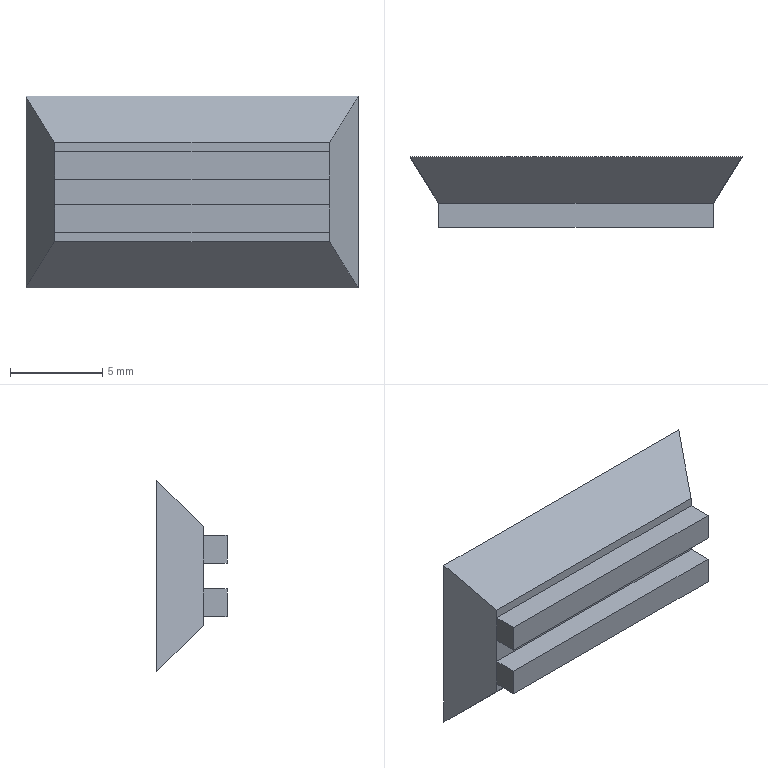Part | STEP file | D4NS_1CF_CAP^D4NS_1CF_Laser guard | 1 solid | 18 faces | box 18 x 3.8 x 10.4 mm | volume 386.227 mm3 | plane 18
STEP:
#1=CARTESIAN_POINT('',(0.,0.,0.));
#2=DIRECTION('',(0.,0.,1.));
#3=DIRECTION('',(1.,0.,0.));
#4=AXIS2_PLACEMENT_3D('',#1,#2,#3);
#5=CARTESIAN_POINT('',(-1.55,-3.8,7.4));
#6=VERTEX_POINT('',#5);
#7=CARTESIAN_POINT('',(-16.45,-3.8,7.4));
#8=VERTEX_POINT('',#7);
#9=CARTESIAN_POINT('',(-16.45,-3.8,7.4));
#10=DIRECTION('',(-1.,0.,0.));
#11=VECTOR('',#10,1.);
#12=LINE('',#9,#11);
#13=CARTESIAN_POINT('',(-1.55,-3.8,7.4));
#14=DIRECTION('',(0.,1.,0.));
#15=DIRECTION('',(1.,0.,0.));
#16=AXIS2_PLACEMENT_3D('',#13,#14,#15);
#17=PLANE('',#16);
#18=CARTESIAN_POINT('',(-14.9,0.));
#19=DIRECTION('',(-1.,0.));
#20=VECTOR('',#19,1.);
#21=LINE('',#18,#20);
#22=(GEOMETRIC_REPRESENTATION_CONTEXT(2)PARAMETRIC_REPRESENTATION_CONTEXT()REPRESENTATION_CONTEXT('',''));
#23=DEFINITIONAL_REPRESENTATION('',(#21),#22);
#24=PCURVE('',#17,#23);
#25=CARTESIAN_POINT('',(-16.45,-3.8,7.4));
#26=DIRECTION('',(0.,0.,-1.));
#27=DIRECTION('',(0.,-1.,0.));
#28=AXIS2_PLACEMENT_3D('',#25,#26,#27);
#29=PLANE('',#28);
#30=CARTESIAN_POINT('',(0.,0.));
#31=DIRECTION('',(0.,1.));
#32=VECTOR('',#31,1.);
#33=LINE('',#30,#32);
#34=(GEOMETRIC_REPRESENTATION_CONTEXT(2)PARAMETRIC_REPRESENTATION_CONTEXT()REPRESENTATION_CONTEXT('',''));
#35=DEFINITIONAL_REPRESENTATION('',(#33),#34);
#36=PCURVE('',#29,#35);
#37=SURFACE_CURVE('',#12,(#24,#36),.PCURVE_S1.);
#38=EDGE_CURVE('',#6,#8,#37,.T.);
#39=ORIENTED_EDGE('',*,*,#38,.T.);
#40=CARTESIAN_POINT('',(-16.45,-3.8,5.9));
#41=VERTEX_POINT('',#40);
#42=CARTESIAN_POINT('',(-16.45,-3.8,7.4));
#43=DIRECTION('',(0.,0.,-1.));
#44=VECTOR('',#43,1.);
#45=LINE('',#42,#44);
#46=CARTESIAN_POINT('',(-14.9,0.));
#47=DIRECTION('',(0.,1.));
#48=VECTOR('',#47,1.);
#49=LINE('',#46,#48);
#50=(GEOMETRIC_REPRESENTATION_CONTEXT(2)PARAMETRIC_REPRESENTATION_CONTEXT()REPRESENTATION_CONTEXT('',''));
#51=DEFINITIONAL_REPRESENTATION('',(#49),#50);
#52=PCURVE('',#17,#51);
#53=CARTESIAN_POINT('',(-16.45,-3.8,7.4));
#54=DIRECTION('',(1.,0.,0.));
#55=DIRECTION('',(0.,1.,0.));
#56=AXIS2_PLACEMENT_3D('',#53,#54,#55);
#57=PLANE('',#56);
#58=CARTESIAN_POINT('',(0.,0.));
#59=DIRECTION('',(0.,-1.));
#60=VECTOR('',#59,1.);
#61=LINE('',#58,#60);
#62=(GEOMETRIC_REPRESENTATION_CONTEXT(2)PARAMETRIC_REPRESENTATION_CONTEXT()REPRESENTATION_CONTEXT('',''));
#63=DEFINITIONAL_REPRESENTATION('',(#61),#62);
#64=PCURVE('',#57,#63);
#65=SURFACE_CURVE('',#45,(#52,#64),.PCURVE_S1.);
#66=EDGE_CURVE('',#8,#41,#65,.T.);
#67=ORIENTED_EDGE('',*,*,#66,.T.);
#68=CARTESIAN_POINT('',(-1.55,-3.8,5.9));
#69=VERTEX_POINT('',#68);
#70=CARTESIAN_POINT('',(-16.45,-3.8,5.9));
#71=DIRECTION('',(1.,0.,0.));
#72=VECTOR('',#71,1.);
#73=LINE('',#70,#72);
#74=CARTESIAN_POINT('',(-14.9,1.5));
#75=DIRECTION('',(1.,0.));
#76=VECTOR('',#75,1.);
#77=LINE('',#74,#76);
#78=(GEOMETRIC_REPRESENTATION_CONTEXT(2)PARAMETRIC_REPRESENTATION_CONTEXT()REPRESENTATION_CONTEXT('',''));
#79=DEFINITIONAL_REPRESENTATION('',(#77),#78);
#80=PCURVE('',#17,#79);
#81=CARTESIAN_POINT('',(-16.45,-3.8,5.9));
#82=DIRECTION('',(0.,0.,1.));
#83=DIRECTION('',(1.,0.,0.));
#84=AXIS2_PLACEMENT_3D('',#81,#82,#83);
#85=PLANE('',#84);
#86=CARTESIAN_POINT('',(0.,0.));
#87=DIRECTION('',(1.,0.));
#88=VECTOR('',#87,1.);
#89=LINE('',#86,#88);
#90=(GEOMETRIC_REPRESENTATION_CONTEXT(2)PARAMETRIC_REPRESENTATION_CONTEXT()REPRESENTATION_CONTEXT('',''));
#91=DEFINITIONAL_REPRESENTATION('',(#89),#90);
#92=PCURVE('',#85,#91);
#93=SURFACE_CURVE('',#73,(#80,#92),.PCURVE_S1.);
#94=EDGE_CURVE('',#41,#69,#93,.T.);
#95=ORIENTED_EDGE('',*,*,#94,.T.);
#96=CARTESIAN_POINT('',(-1.55,-3.8,7.4));
#97=DIRECTION('',(0.,0.,1.));
#98=VECTOR('',#97,1.);
#99=LINE('',#96,#98);
#100=CARTESIAN_POINT('',(0.,0.));
#101=DIRECTION('',(0.,-1.));
#102=VECTOR('',#101,1.);
#103=LINE('',#100,#102);
#104=(GEOMETRIC_REPRESENTATION_CONTEXT(2)PARAMETRIC_REPRESENTATION_CONTEXT()REPRESENTATION_CONTEXT('',''));
#105=DEFINITIONAL_REPRESENTATION('',(#103),#104);
#106=PCURVE('',#17,#105);
#107=CARTESIAN_POINT('',(-1.55,-3.8,7.4));
#108=DIRECTION('',(-1.,0.,0.));
#109=DIRECTION('',(0.,0.,1.));
#110=AXIS2_PLACEMENT_3D('',#107,#108,#109);
#111=PLANE('',#110);
#112=CARTESIAN_POINT('',(0.,0.));
#113=DIRECTION('',(1.,0.));
#114=VECTOR('',#113,1.);
#115=LINE('',#112,#114);
#116=(GEOMETRIC_REPRESENTATION_CONTEXT(2)PARAMETRIC_REPRESENTATION_CONTEXT()REPRESENTATION_CONTEXT('',''));
#117=DEFINITIONAL_REPRESENTATION('',(#115),#116);
#118=PCURVE('',#111,#117);
#119=SURFACE_CURVE('',#99,(#106,#118),.PCURVE_S1.);
#120=EDGE_CURVE('',#69,#6,#119,.T.);
#121=ORIENTED_EDGE('',*,*,#120,.T.);
#122=EDGE_LOOP('',(#39,#67,#95,#121));
#123=FACE_BOUND('',#122,.T.);
#124=ADVANCED_FACE('',(#123),#17,.F.);
#125=CARTESIAN_POINT('',(-1.55,-2.5,7.4));
#126=VERTEX_POINT('',#125);
#127=CARTESIAN_POINT('',(-16.45,-2.5,7.4));
#128=VERTEX_POINT('',#127);
#129=CARTESIAN_POINT('',(-16.45,-2.5,7.4));
#130=DIRECTION('',(-1.,0.,0.));
#131=VECTOR('',#130,1.);
#132=LINE('',#129,#131);
#133=CARTESIAN_POINT('',(-1.3,0.));
#134=DIRECTION('',(0.,1.));
#135=VECTOR('',#134,1.);
#136=LINE('',#133,#135);
#137=(GEOMETRIC_REPRESENTATION_CONTEXT(2)PARAMETRIC_REPRESENTATION_CONTEXT()REPRESENTATION_CONTEXT('',''));
#138=DEFINITIONAL_REPRESENTATION('',(#136),#137);
#139=PCURVE('',#29,#138);
#140=CARTESIAN_POINT('',(0.,-2.5,0.));
#141=DIRECTION('',(0.,-1.,0.));
#142=DIRECTION('',(0.,0.,-1.));
#143=AXIS2_PLACEMENT_3D('',#140,#141,#142);
#144=PLANE('',#143);
#145=CARTESIAN_POINT('',(-7.4,-16.45));
#146=DIRECTION('',(0.,-1.));
#147=VECTOR('',#146,1.);
#148=LINE('',#145,#147);
#149=(GEOMETRIC_REPRESENTATION_CONTEXT(2)PARAMETRIC_REPRESENTATION_CONTEXT()REPRESENTATION_CONTEXT('',''));
#150=DEFINITIONAL_REPRESENTATION('',(#148),#149);
#151=PCURVE('',#144,#150);
#152=SURFACE_CURVE('',#132,(#139,#151),.PCURVE_S1.);
#153=EDGE_CURVE('',#126,#128,#152,.T.);
#154=ORIENTED_EDGE('',*,*,#153,.T.);
#155=CARTESIAN_POINT('',(-16.45,-3.8,7.4));
#156=DIRECTION('',(0.,1.,0.));
#157=VECTOR('',#156,1.);
#158=LINE('',#155,#157);
#159=CARTESIAN_POINT('',(0.,0.));
#160=DIRECTION('',(-1.,0.));
#161=VECTOR('',#160,1.);
#162=LINE('',#159,#161);
#163=(GEOMETRIC_REPRESENTATION_CONTEXT(2)PARAMETRIC_REPRESENTATION_CONTEXT()REPRESENTATION_CONTEXT('',''));
#164=DEFINITIONAL_REPRESENTATION('',(#162),#163);
#165=PCURVE('',#29,#164);
#166=CARTESIAN_POINT('',(0.,0.));
#167=DIRECTION('',(1.,0.));
#168=VECTOR('',#167,1.);
#169=LINE('',#166,#168);
#170=(GEOMETRIC_REPRESENTATION_CONTEXT(2)PARAMETRIC_REPRESENTATION_CONTEXT()REPRESENTATION_CONTEXT('',''));
#171=DEFINITIONAL_REPRESENTATION('',(#169),#170);
#172=PCURVE('',#57,#171);
#173=SURFACE_CURVE('',#158,(#165,#172),.PCURVE_S1.);
#174=EDGE_CURVE('',#8,#128,#173,.T.);
#175=ORIENTED_EDGE('',*,*,#174,.F.);
#176=ORIENTED_EDGE('',*,*,#38,.F.);
#177=CARTESIAN_POINT('',(-1.55,-3.8,7.4));
#178=DIRECTION('',(0.,1.,0.));
#179=VECTOR('',#178,1.);
#180=LINE('',#177,#179);
#181=CARTESIAN_POINT('',(0.,-14.9));
#182=DIRECTION('',(-1.,0.));
#183=VECTOR('',#182,1.);
#184=LINE('',#181,#183);
#185=(GEOMETRIC_REPRESENTATION_CONTEXT(2)PARAMETRIC_REPRESENTATION_CONTEXT()REPRESENTATION_CONTEXT('',''));
#186=DEFINITIONAL_REPRESENTATION('',(#184),#185);
#187=PCURVE('',#29,#186);
#188=CARTESIAN_POINT('',(0.,0.));
#189=DIRECTION('',(0.,1.));
#190=VECTOR('',#189,1.);
#191=LINE('',#188,#190);
#192=(GEOMETRIC_REPRESENTATION_CONTEXT(2)PARAMETRIC_REPRESENTATION_CONTEXT()REPRESENTATION_CONTEXT('',''));
#193=DEFINITIONAL_REPRESENTATION('',(#191),#192);
#194=PCURVE('',#111,#193);
#195=SURFACE_CURVE('',#180,(#187,#194),.PCURVE_S1.);
#196=EDGE_CURVE('',#6,#126,#195,.T.);
#197=ORIENTED_EDGE('',*,*,#196,.T.);
#198=EDGE_LOOP('',(#154,#175,#176,#197));
#199=FACE_BOUND('',#198,.T.);
#200=ADVANCED_FACE('',(#199),#29,.F.);
#201=CARTESIAN_POINT('',(-16.45,-2.5,5.9));
#202=VERTEX_POINT('',#201);
#203=CARTESIAN_POINT('',(-1.55,-2.5,5.9));
#204=VERTEX_POINT('',#203);
#205=CARTESIAN_POINT('',(-16.45,-2.5,5.9));
#206=DIRECTION('',(1.,0.,0.));
#207=VECTOR('',#206,1.);
#208=LINE('',#205,#207);
#209=CARTESIAN_POINT('',(0.,1.3));
#210=DIRECTION('',(1.,0.));
#211=VECTOR('',#210,1.);
#212=LINE('',#209,#211);
#213=(GEOMETRIC_REPRESENTATION_CONTEXT(2)PARAMETRIC_REPRESENTATION_CONTEXT()REPRESENTATION_CONTEXT('',''));
#214=DEFINITIONAL_REPRESENTATION('',(#212),#213);
#215=PCURVE('',#85,#214);
#216=CARTESIAN_POINT('',(0.,-2.5,0.));
#217=DIRECTION('',(0.,-1.,0.));
#218=DIRECTION('',(0.,0.,-1.));
#219=AXIS2_PLACEMENT_3D('',#216,#217,#218);
#220=PLANE('',#219);
#221=CARTESIAN_POINT('',(-5.9,-16.45));
#222=DIRECTION('',(0.,1.));
#223=VECTOR('',#222,1.);
#224=LINE('',#221,#223);
#225=(GEOMETRIC_REPRESENTATION_CONTEXT(2)PARAMETRIC_REPRESENTATION_CONTEXT()REPRESENTATION_CONTEXT('',''));
#226=DEFINITIONAL_REPRESENTATION('',(#224),#225);
#227=PCURVE('',#220,#226);
#228=SURFACE_CURVE('',#208,(#215,#227),.PCURVE_S1.);
#229=EDGE_CURVE('',#202,#204,#228,.T.);
#230=ORIENTED_EDGE('',*,*,#229,.T.);
#231=CARTESIAN_POINT('',(-1.55,-3.8,5.9));
#232=DIRECTION('',(0.,1.,0.));
#233=VECTOR('',#232,1.);
#234=LINE('',#231,#233);
#235=CARTESIAN_POINT('',(14.9,0.));
#236=DIRECTION('',(0.,1.));
#237=VECTOR('',#236,1.);
#238=LINE('',#235,#237);
#239=(GEOMETRIC_REPRESENTATION_CONTEXT(2)PARAMETRIC_REPRESENTATION_CONTEXT()REPRESENTATION_CONTEXT('',''));
#240=DEFINITIONAL_REPRESENTATION('',(#238),#239);
#241=PCURVE('',#85,#240);
#242=CARTESIAN_POINT('',(-1.5,0.));
#243=DIRECTION('',(0.,1.));
#244=VECTOR('',#243,1.);
#245=LINE('',#242,#244);
#246=(GEOMETRIC_REPRESENTATION_CONTEXT(2)PARAMETRIC_REPRESENTATION_CONTEXT()REPRESENTATION_CONTEXT('',''));
#247=DEFINITIONAL_REPRESENTATION('',(#245),#246);
#248=PCURVE('',#111,#247);
#249=SURFACE_CURVE('',#234,(#241,#248),.PCURVE_S1.);
#250=EDGE_CURVE('',#69,#204,#249,.T.);
#251=ORIENTED_EDGE('',*,*,#250,.F.);
#252=ORIENTED_EDGE('',*,*,#94,.F.);
#253=CARTESIAN_POINT('',(-16.45,-3.8,5.9));
#254=DIRECTION('',(0.,1.,0.));
#255=VECTOR('',#254,1.);
#256=LINE('',#253,#255);
#257=CARTESIAN_POINT('',(0.,0.));
#258=DIRECTION('',(0.,1.));
#259=VECTOR('',#258,1.);
#260=LINE('',#257,#259);
#261=(GEOMETRIC_REPRESENTATION_CONTEXT(2)PARAMETRIC_REPRESENTATION_CONTEXT()REPRESENTATION_CONTEXT('',''));
#262=DEFINITIONAL_REPRESENTATION('',(#260),#261);
#263=PCURVE('',#85,#262);
#264=CARTESIAN_POINT('',(0.,-1.5));
#265=DIRECTION('',(1.,0.));
#266=VECTOR('',#265,1.);
#267=LINE('',#264,#266);
#268=(GEOMETRIC_REPRESENTATION_CONTEXT(2)PARAMETRIC_REPRESENTATION_CONTEXT()REPRESENTATION_CONTEXT('',''));
#269=DEFINITIONAL_REPRESENTATION('',(#267),#268);
#270=PCURVE('',#57,#269);
#271=SURFACE_CURVE('',#256,(#263,#270),.PCURVE_S1.);
#272=EDGE_CURVE('',#41,#202,#271,.T.);
#273=ORIENTED_EDGE('',*,*,#272,.T.);
#274=EDGE_LOOP('',(#230,#251,#252,#273));
#275=FACE_BOUND('',#274,.T.);
#276=ADVANCED_FACE('',(#275),#85,.F.);
#277=CARTESIAN_POINT('',(-1.55,-2.5,7.4));
#278=DIRECTION('',(0.,0.,1.));
#279=VECTOR('',#278,1.);
#280=LINE('',#277,#279);
#281=CARTESIAN_POINT('',(0.,1.3));
#282=DIRECTION('',(1.,0.));
#283=VECTOR('',#282,1.);
#284=LINE('',#281,#283);
#285=(GEOMETRIC_REPRESENTATION_CONTEXT(2)PARAMETRIC_REPRESENTATION_CONTEXT()REPRESENTATION_CONTEXT('',''));
#286=DEFINITIONAL_REPRESENTATION('',(#284),#285);
#287=PCURVE('',#111,#286);
#288=CARTESIAN_POINT('',(0.,0.,0.));
#289=DIRECTION('',(-0.8499,0.5269,0.));
#290=DIRECTION('',(0.,0.,1.));
#291=AXIS2_PLACEMENT_3D('',#288,#289,#290);
#292=PLANE('',#291);
#293=CARTESIAN_POINT('',(7.4,-2.942));
#294=DIRECTION('',(1.,0.));
#295=VECTOR('',#294,1.);
#296=LINE('',#293,#295);
#297=(GEOMETRIC_REPRESENTATION_CONTEXT(2)PARAMETRIC_REPRESENTATION_CONTEXT()REPRESENTATION_CONTEXT('',''));
#298=DEFINITIONAL_REPRESENTATION('',(#296),#297);
#299=PCURVE('',#292,#298);
#300=SURFACE_CURVE('',#280,(#287,#299),.PCURVE_S1.);
#301=EDGE_CURVE('',#204,#126,#300,.T.);
#302=ORIENTED_EDGE('',*,*,#301,.T.);
#303=ORIENTED_EDGE('',*,*,#196,.F.);
#304=ORIENTED_EDGE('',*,*,#120,.F.);
#305=ORIENTED_EDGE('',*,*,#250,.T.);
#306=EDGE_LOOP('',(#302,#303,#304,#305));
#307=FACE_BOUND('',#306,.T.);
#308=ADVANCED_FACE('',(#307),#111,.F.);
#309=CARTESIAN_POINT('',(-16.45,-2.5,7.9));
#310=VERTEX_POINT('',#309);
#311=CARTESIAN_POINT('',(-18.,0.,10.4));
#312=VERTEX_POINT('',#311);
#313=CARTESIAN_POINT('',(-15.296,-4.362,6.038));
#314=DIRECTION('',(-0.4015,0.6476,0.6476));
#315=VECTOR('',#314,1.);
#316=LINE('',#313,#315);
#317=CARTESIAN_POINT('',(0.,0.,10.4));
#318=DIRECTION('',(0.,0.7071,-0.7071));
#319=DIRECTION('',(-1.,0.,0.));
#320=AXIS2_PLACEMENT_3D('',#317,#318,#319);
#321=PLANE('',#320);
#322=CARTESIAN_POINT('',(15.296,-6.168));
#323=DIRECTION('',(0.4015,0.9159));
#324=VECTOR('',#323,1.);
#325=LINE('',#322,#324);
#326=(GEOMETRIC_REPRESENTATION_CONTEXT(2)PARAMETRIC_REPRESENTATION_CONTEXT()REPRESENTATION_CONTEXT('',''));
#327=DEFINITIONAL_REPRESENTATION('',(#325),#326);
#328=PCURVE('',#321,#327);
#329=CARTESIAN_POINT('',(-18.,0.,0.));
#330=DIRECTION('',(0.8499,0.5269,0.));
#331=DIRECTION('',(0.,0.,-1.));
#332=AXIS2_PLACEMENT_3D('',#329,#330,#331);
#333=PLANE('',#332);
#334=CARTESIAN_POINT('',(-6.038,-5.132));
#335=DIRECTION('',(-0.6476,0.762));
#336=VECTOR('',#335,1.);
#337=LINE('',#334,#336);
#338=(GEOMETRIC_REPRESENTATION_CONTEXT(2)PARAMETRIC_REPRESENTATION_CONTEXT()REPRESENTATION_CONTEXT('',''));
#339=DEFINITIONAL_REPRESENTATION('',(#337),#338);
#340=PCURVE('',#333,#339);
#341=SURFACE_CURVE('',#316,(#328,#340),.PCURVE_S1.);
#342=EDGE_CURVE('',#310,#312,#341,.T.);
#343=ORIENTED_EDGE('',*,*,#342,.F.);
#344=CARTESIAN_POINT('',(-1.55,-2.5,7.9));
#345=VERTEX_POINT('',#344);
#346=CARTESIAN_POINT('',(0.,-2.5,7.9));
#347=DIRECTION('',(-1.,0.,0.));
#348=VECTOR('',#347,1.);
#349=LINE('',#346,#348);
#350=CARTESIAN_POINT('',(0.,-3.536));
#351=DIRECTION('',(1.,0.));
#352=VECTOR('',#351,1.);
#353=LINE('',#350,#352);
#354=(GEOMETRIC_REPRESENTATION_CONTEXT(2)PARAMETRIC_REPRESENTATION_CONTEXT()REPRESENTATION_CONTEXT('',''));
#355=DEFINITIONAL_REPRESENTATION('',(#353),#354);
#356=PCURVE('',#321,#355);
#357=CARTESIAN_POINT('',(-7.9,0.));
#358=DIRECTION('',(0.,-1.));
#359=VECTOR('',#358,1.);
#360=LINE('',#357,#359);
#361=(GEOMETRIC_REPRESENTATION_CONTEXT(2)PARAMETRIC_REPRESENTATION_CONTEXT()REPRESENTATION_CONTEXT('',''));
#362=DEFINITIONAL_REPRESENTATION('',(#360),#361);
#363=PCURVE('',#144,#362);
#364=SURFACE_CURVE('',#349,(#356,#363),.PCURVE_S1.);
#365=EDGE_CURVE('',#345,#310,#364,.T.);
#366=ORIENTED_EDGE('',*,*,#365,.F.);
#367=CARTESIAN_POINT('',(0.,0.,10.4));
#368=VERTEX_POINT('',#367);
#369=CARTESIAN_POINT('',(-2.704,-4.362,6.038));
#370=DIRECTION('',(-0.4015,-0.6476,-0.6476));
#371=VECTOR('',#370,1.);
#372=LINE('',#369,#371);
#373=CARTESIAN_POINT('',(2.704,-6.168));
#374=DIRECTION('',(0.4015,-0.9159));
#375=VECTOR('',#374,1.);
#376=LINE('',#373,#375);
#377=(GEOMETRIC_REPRESENTATION_CONTEXT(2)PARAMETRIC_REPRESENTATION_CONTEXT()REPRESENTATION_CONTEXT('',''));
#378=DEFINITIONAL_REPRESENTATION('',(#376),#377);
#379=PCURVE('',#321,#378);
#380=CARTESIAN_POINT('',(6.038,-5.132));
#381=DIRECTION('',(-0.6476,-0.762));
#382=VECTOR('',#381,1.);
#383=LINE('',#380,#382);
#384=(GEOMETRIC_REPRESENTATION_CONTEXT(2)PARAMETRIC_REPRESENTATION_CONTEXT()REPRESENTATION_CONTEXT('',''));
#385=DEFINITIONAL_REPRESENTATION('',(#383),#384);
#386=PCURVE('',#292,#385);
#387=SURFACE_CURVE('',#372,(#379,#386),.PCURVE_S1.);
#388=EDGE_CURVE('',#368,#345,#387,.T.);
#389=ORIENTED_EDGE('',*,*,#388,.F.);
#390=CARTESIAN_POINT('',(0.,0.,10.4));
#391=DIRECTION('',(1.,0.,0.));
#392=VECTOR('',#391,1.);
#393=LINE('',#390,#392);
#394=CARTESIAN_POINT('',(0.,0.));
#395=DIRECTION('',(-1.,0.));
#396=VECTOR('',#395,1.);
#397=LINE('',#394,#396);
#398=(GEOMETRIC_REPRESENTATION_CONTEXT(2)PARAMETRIC_REPRESENTATION_CONTEXT()REPRESENTATION_CONTEXT('',''));
#399=DEFINITIONAL_REPRESENTATION('',(#397),#398);
#400=PCURVE('',#321,#399);
#401=CARTESIAN_POINT('',(0.,0.,0.));
#402=DIRECTION('',(0.,-1.,0.));
#403=DIRECTION('',(0.,0.,-1.));
#404=AXIS2_PLACEMENT_3D('',#401,#402,#403);
#405=PLANE('',#404);
#406=CARTESIAN_POINT('',(-10.4,0.));
#407=DIRECTION('',(0.,1.));
#408=VECTOR('',#407,1.);
#409=LINE('',#406,#408);
#410=(GEOMETRIC_REPRESENTATION_CONTEXT(2)PARAMETRIC_REPRESENTATION_CONTEXT()REPRESENTATION_CONTEXT('',''));
#411=DEFINITIONAL_REPRESENTATION('',(#409),#410);
#412=PCURVE('',#405,#411);
#413=SURFACE_CURVE('',#393,(#400,#412),.PCURVE_S1.);
#414=EDGE_CURVE('',#312,#368,#413,.T.);
#415=ORIENTED_EDGE('',*,*,#414,.F.);
#416=EDGE_LOOP('',(#343,#366,#389,#415));
#417=FACE_BOUND('',#416,.T.);
#418=ADVANCED_FACE('',(#417),#321,.F.);
#419=CARTESIAN_POINT('',(0.,0.,0.));
#420=VERTEX_POINT('',#419);
#421=CARTESIAN_POINT('',(0.,0.,0.));
#422=DIRECTION('',(0.,0.,-1.));
#423=VECTOR('',#422,1.);
#424=LINE('',#421,#423);
#425=CARTESIAN_POINT('',(0.,0.));
#426=DIRECTION('',(1.,0.));
#427=VECTOR('',#426,1.);
#428=LINE('',#425,#427);
#429=(GEOMETRIC_REPRESENTATION_CONTEXT(2)PARAMETRIC_REPRESENTATION_CONTEXT()REPRESENTATION_CONTEXT('',''));
#430=DEFINITIONAL_REPRESENTATION('',(#428),#429);
#431=PCURVE('',#405,#430);
#432=CARTESIAN_POINT('',(0.,0.));
#433=DIRECTION('',(-1.,0.));
#434=VECTOR('',#433,1.);
#435=LINE('',#432,#434);
#436=(GEOMETRIC_REPRESENTATION_CONTEXT(2)PARAMETRIC_REPRESENTATION_CONTEXT()REPRESENTATION_CONTEXT('',''));
#437=DEFINITIONAL_REPRESENTATION('',(#435),#436);
#438=PCURVE('',#292,#437);
#439=SURFACE_CURVE('',#424,(#431,#438),.PCURVE_S1.);
#440=EDGE_CURVE('',#368,#420,#439,.T.);
#441=ORIENTED_EDGE('',*,*,#440,.T.);
#442=CARTESIAN_POINT('',(-18.,0.,0.));
#443=VERTEX_POINT('',#442);
#444=CARTESIAN_POINT('',(0.,0.,0.));
#445=DIRECTION('',(-1.,0.,0.));
#446=VECTOR('',#445,1.);
#447=LINE('',#444,#446);
#448=CARTESIAN_POINT('',(0.,0.));
#449=DIRECTION('',(0.,-1.));
#450=VECTOR('',#449,1.);
#451=LINE('',#448,#450);
#452=(GEOMETRIC_REPRESENTATION_CONTEXT(2)PARAMETRIC_REPRESENTATION_CONTEXT()REPRESENTATION_CONTEXT('',''));
#453=DEFINITIONAL_REPRESENTATION('',(#451),#452);
#454=PCURVE('',#405,#453);
#455=CARTESIAN_POINT('',(0.,0.,0.));
#456=DIRECTION('',(0.,0.7071,0.7071));
#457=DIRECTION('',(1.,0.,0.));
#458=AXIS2_PLACEMENT_3D('',#455,#456,#457);
#459=PLANE('',#458);
#460=CARTESIAN_POINT('',(0.,0.));
#461=DIRECTION('',(-1.,0.));
#462=VECTOR('',#461,1.);
#463=LINE('',#460,#462);
#464=(GEOMETRIC_REPRESENTATION_CONTEXT(2)PARAMETRIC_REPRESENTATION_CONTEXT()REPRESENTATION_CONTEXT('',''));
#465=DEFINITIONAL_REPRESENTATION('',(#463),#464);
#466=PCURVE('',#459,#465);
#467=SURFACE_CURVE('',#447,(#454,#466),.PCURVE_S1.);
#468=EDGE_CURVE('',#420,#443,#467,.T.);
#469=ORIENTED_EDGE('',*,*,#468,.T.);
#470=CARTESIAN_POINT('',(-18.,0.,0.));
#471=DIRECTION('',(0.,0.,1.));
#472=VECTOR('',#471,1.);
#473=LINE('',#470,#472);
#474=CARTESIAN_POINT('',(0.,-18.));
#475=DIRECTION('',(-1.,0.));
#476=VECTOR('',#475,1.);
#477=LINE('',#474,#476);
#478=(GEOMETRIC_REPRESENTATION_CONTEXT(2)PARAMETRIC_REPRESENTATION_CONTEXT()REPRESENTATION_CONTEXT('',''));
#479=DEFINITIONAL_REPRESENTATION('',(#477),#478);
#480=PCURVE('',#405,#479);
#481=CARTESIAN_POINT('',(0.,0.));
#482=DIRECTION('',(-1.,0.));
#483=VECTOR('',#482,1.);
#484=LINE('',#481,#483);
#485=(GEOMETRIC_REPRESENTATION_CONTEXT(2)PARAMETRIC_REPRESENTATION_CONTEXT()REPRESENTATION_CONTEXT('',''));
#486=DEFINITIONAL_REPRESENTATION('',(#484),#485);
#487=PCURVE('',#333,#486);
#488=SURFACE_CURVE('',#473,(#480,#487),.PCURVE_S1.);
#489=EDGE_CURVE('',#443,#312,#488,.T.);
#490=ORIENTED_EDGE('',*,*,#489,.T.);
#491=ORIENTED_EDGE('',*,*,#414,.T.);
#492=EDGE_LOOP('',(#441,#469,#490,#491));
#493=FACE_BOUND('',#492,.T.);
#494=ADVANCED_FACE('',(#493),#405,.F.);
#495=CARTESIAN_POINT('',(-16.45,-2.5,7.4));
#496=DIRECTION('',(0.,0.,-1.));
#497=VECTOR('',#496,1.);
#498=LINE('',#495,#497);
#499=CARTESIAN_POINT('',(1.3,0.));
#500=DIRECTION('',(0.,-1.));
#501=VECTOR('',#500,1.);
#502=LINE('',#499,#501);
#503=(GEOMETRIC_REPRESENTATION_CONTEXT(2)PARAMETRIC_REPRESENTATION_CONTEXT()REPRESENTATION_CONTEXT('',''));
#504=DEFINITIONAL_REPRESENTATION('',(#502),#503);
#505=PCURVE('',#57,#504);
#506=CARTESIAN_POINT('',(-7.4,-2.942));
#507=DIRECTION('',(1.,0.));
#508=VECTOR('',#507,1.);
#509=LINE('',#506,#508);
#510=(GEOMETRIC_REPRESENTATION_CONTEXT(2)PARAMETRIC_REPRESENTATION_CONTEXT()REPRESENTATION_CONTEXT('',''));
#511=DEFINITIONAL_REPRESENTATION('',(#509),#510);
#512=PCURVE('',#333,#511);
#513=SURFACE_CURVE('',#498,(#505,#512),.PCURVE_S1.);
#514=EDGE_CURVE('',#128,#202,#513,.T.);
#515=ORIENTED_EDGE('',*,*,#514,.T.);
#516=ORIENTED_EDGE('',*,*,#272,.F.);
#517=ORIENTED_EDGE('',*,*,#66,.F.);
#518=ORIENTED_EDGE('',*,*,#174,.T.);
#519=EDGE_LOOP('',(#515,#516,#517,#518));
#520=FACE_BOUND('',#519,.T.);
#521=ADVANCED_FACE('',(#520),#57,.F.);
#522=CARTESIAN_POINT('',(-1.55,-2.5,0.));
#523=DIRECTION('',(0.,0.,1.));
#524=VECTOR('',#523,1.);
#525=LINE('',#522,#524);
#526=CARTESIAN_POINT('',(0.,-1.55));
#527=DIRECTION('',(-1.,0.));
#528=VECTOR('',#527,1.);
#529=LINE('',#526,#528);
#530=(GEOMETRIC_REPRESENTATION_CONTEXT(2)PARAMETRIC_REPRESENTATION_CONTEXT()REPRESENTATION_CONTEXT('',''));
#531=DEFINITIONAL_REPRESENTATION('',(#529),#530);
#532=PCURVE('',#144,#531);
#533=CARTESIAN_POINT('',(0.,-2.942));
#534=DIRECTION('',(1.,0.));
#535=VECTOR('',#534,1.);
#536=LINE('',#533,#535);
#537=(GEOMETRIC_REPRESENTATION_CONTEXT(2)PARAMETRIC_REPRESENTATION_CONTEXT()REPRESENTATION_CONTEXT('',''));
#538=DEFINITIONAL_REPRESENTATION('',(#536),#537);
#539=PCURVE('',#292,#538);
#540=SURFACE_CURVE('',#525,(#532,#539),.PCURVE_S1.);
#541=EDGE_CURVE('',#126,#345,#540,.T.);
#542=ORIENTED_EDGE('',*,*,#541,.T.);
#543=ORIENTED_EDGE('',*,*,#365,.T.);
#544=CARTESIAN_POINT('',(-16.45,-2.5,0.));
#545=DIRECTION('',(0.,0.,-1.));
#546=VECTOR('',#545,1.);
#547=LINE('',#544,#546);
#548=CARTESIAN_POINT('',(0.,-16.45));
#549=DIRECTION('',(1.,0.));
#550=VECTOR('',#549,1.);
#551=LINE('',#548,#550);
#552=(GEOMETRIC_REPRESENTATION_CONTEXT(2)PARAMETRIC_REPRESENTATION_CONTEXT()REPRESENTATION_CONTEXT('',''));
#553=DEFINITIONAL_REPRESENTATION('',(#551),#552);
#554=PCURVE('',#144,#553);
#555=CARTESIAN_POINT('',(0.,-2.942));
#556=DIRECTION('',(1.,0.));
#557=VECTOR('',#556,1.);
#558=LINE('',#555,#557);
#559=(GEOMETRIC_REPRESENTATION_CONTEXT(2)PARAMETRIC_REPRESENTATION_CONTEXT()REPRESENTATION_CONTEXT('',''));
#560=DEFINITIONAL_REPRESENTATION('',(#558),#559);
#561=PCURVE('',#333,#560);
#562=SURFACE_CURVE('',#547,(#554,#561),.PCURVE_S1.);
#563=EDGE_CURVE('',#310,#128,#562,.T.);
#564=ORIENTED_EDGE('',*,*,#563,.T.);
#565=ORIENTED_EDGE('',*,*,#153,.F.);
#566=EDGE_LOOP('',(#542,#543,#564,#565));
#567=FACE_BOUND('',#566,.T.);
#568=ADVANCED_FACE('',(#567),#144,.T.);
#569=ORIENTED_EDGE('',*,*,#229,.F.);
#570=CARTESIAN_POINT('',(-16.45,-2.5,4.5));
#571=VERTEX_POINT('',#570);
#572=CARTESIAN_POINT('',(-16.45,-2.5,0.));
#573=DIRECTION('',(0.,0.,-1.));
#574=VECTOR('',#573,1.);
#575=LINE('',#572,#574);
#576=CARTESIAN_POINT('',(0.,-16.45));
#577=DIRECTION('',(1.,0.));
#578=VECTOR('',#577,1.);
#579=LINE('',#576,#578);
#580=(GEOMETRIC_REPRESENTATION_CONTEXT(2)PARAMETRIC_REPRESENTATION_CONTEXT()REPRESENTATION_CONTEXT('',''));
#581=DEFINITIONAL_REPRESENTATION('',(#579),#580);
#582=PCURVE('',#220,#581);
#583=CARTESIAN_POINT('',(0.,-2.942));
#584=DIRECTION('',(1.,0.));
#585=VECTOR('',#584,1.);
#586=LINE('',#583,#585);
#587=(GEOMETRIC_REPRESENTATION_CONTEXT(2)PARAMETRIC_REPRESENTATION_CONTEXT()REPRESENTATION_CONTEXT('',''));
#588=DEFINITIONAL_REPRESENTATION('',(#586),#587);
#589=PCURVE('',#333,#588);
#590=SURFACE_CURVE('',#575,(#582,#589),.PCURVE_S1.);
#591=EDGE_CURVE('',#202,#571,#590,.T.);
#592=ORIENTED_EDGE('',*,*,#591,.T.);
#593=CARTESIAN_POINT('',(-1.55,-2.5,4.5));
#594=VERTEX_POINT('',#593);
#595=CARTESIAN_POINT('',(-16.45,-2.5,4.5));
#596=DIRECTION('',(-1.,0.,0.));
#597=VECTOR('',#596,1.);
#598=LINE('',#595,#597);
#599=CARTESIAN_POINT('',(-4.5,-16.45));
#600=DIRECTION('',(0.,-1.));
#601=VECTOR('',#600,1.);
#602=LINE('',#599,#601);
#603=(GEOMETRIC_REPRESENTATION_CONTEXT(2)PARAMETRIC_REPRESENTATION_CONTEXT()REPRESENTATION_CONTEXT('',''));
#604=DEFINITIONAL_REPRESENTATION('',(#602),#603);
#605=PCURVE('',#220,#604);
#606=CARTESIAN_POINT('',(-16.45,-3.8,4.5));
#607=DIRECTION('',(0.,0.,-1.));
#608=DIRECTION('',(0.,-1.,0.));
#609=AXIS2_PLACEMENT_3D('',#606,#607,#608);
#610=PLANE('',#609);
#611=CARTESIAN_POINT('',(-1.3,0.));
#612=DIRECTION('',(0.,1.));
#613=VECTOR('',#612,1.);
#614=LINE('',#611,#613);
#615=(GEOMETRIC_REPRESENTATION_CONTEXT(2)PARAMETRIC_REPRESENTATION_CONTEXT()REPRESENTATION_CONTEXT('',''));
#616=DEFINITIONAL_REPRESENTATION('',(#614),#615);
#617=PCURVE('',#610,#616);
#618=SURFACE_CURVE('',#598,(#605,#617),.PCURVE_S1.);
#619=EDGE_CURVE('',#594,#571,#618,.T.);
#620=ORIENTED_EDGE('',*,*,#619,.F.);
#621=CARTESIAN_POINT('',(-1.55,-2.5,0.));
#622=DIRECTION('',(0.,0.,1.));
#623=VECTOR('',#622,1.);
#624=LINE('',#621,#623);
#625=CARTESIAN_POINT('',(0.,-1.55));
#626=DIRECTION('',(-1.,0.));
#627=VECTOR('',#626,1.);
#628=LINE('',#625,#627);
#629=(GEOMETRIC_REPRESENTATION_CONTEXT(2)PARAMETRIC_REPRESENTATION_CONTEXT()REPRESENTATION_CONTEXT('',''));
#630=DEFINITIONAL_REPRESENTATION('',(#628),#629);
#631=PCURVE('',#220,#630);
#632=CARTESIAN_POINT('',(0.,-2.942));
#633=DIRECTION('',(1.,0.));
#634=VECTOR('',#633,1.);
#635=LINE('',#632,#634);
#636=(GEOMETRIC_REPRESENTATION_CONTEXT(2)PARAMETRIC_REPRESENTATION_CONTEXT()REPRESENTATION_CONTEXT('',''));
#637=DEFINITIONAL_REPRESENTATION('',(#635),#636);
#638=PCURVE('',#292,#637);
#639=SURFACE_CURVE('',#624,(#631,#638),.PCURVE_S1.);
#640=EDGE_CURVE('',#594,#204,#639,.T.);
#641=ORIENTED_EDGE('',*,*,#640,.T.);
#642=EDGE_LOOP('',(#569,#592,#620,#641));
#643=FACE_BOUND('',#642,.T.);
#644=ADVANCED_FACE('',(#643),#220,.T.);
#645=CARTESIAN_POINT('',(-1.55,-2.5,2.5));
#646=VERTEX_POINT('',#645);
#647=CARTESIAN_POINT('',(0.,0.,0.));
#648=DIRECTION('',(0.4015,0.6476,-0.6476));
#649=VECTOR('',#648,1.);
#650=LINE('',#647,#649);
#651=CARTESIAN_POINT('',(0.,0.));
#652=DIRECTION('',(0.4015,0.9159));
#653=VECTOR('',#652,1.);
#654=LINE('',#651,#653);
#655=(GEOMETRIC_REPRESENTATION_CONTEXT(2)PARAMETRIC_REPRESENTATION_CONTEXT()REPRESENTATION_CONTEXT('',''));
#656=DEFINITIONAL_REPRESENTATION('',(#654),#655);
#657=PCURVE('',#459,#656);
#658=CARTESIAN_POINT('',(0.,0.));
#659=DIRECTION('',(-0.6476,0.762));
#660=VECTOR('',#659,1.);
#661=LINE('',#658,#660);
#662=(GEOMETRIC_REPRESENTATION_CONTEXT(2)PARAMETRIC_REPRESENTATION_CONTEXT()REPRESENTATION_CONTEXT('',''));
#663=DEFINITIONAL_REPRESENTATION('',(#661),#662);
#664=PCURVE('',#292,#663);
#665=SURFACE_CURVE('',#650,(#657,#664),.PCURVE_S1.);
#666=EDGE_CURVE('',#646,#420,#665,.T.);
#667=ORIENTED_EDGE('',*,*,#666,.F.);
#668=CARTESIAN_POINT('',(-16.45,-2.5,2.5));
#669=VERTEX_POINT('',#668);
#670=CARTESIAN_POINT('',(0.,-2.5,2.5));
#671=DIRECTION('',(1.,0.,0.));
#672=VECTOR('',#671,1.);
#673=LINE('',#670,#672);
#674=CARTESIAN_POINT('',(0.,-3.536));
#675=DIRECTION('',(1.,0.));
#676=VECTOR('',#675,1.);
#677=LINE('',#674,#676);
#678=(GEOMETRIC_REPRESENTATION_CONTEXT(2)PARAMETRIC_REPRESENTATION_CONTEXT()REPRESENTATION_CONTEXT('',''));
#679=DEFINITIONAL_REPRESENTATION('',(#677),#678);
#680=PCURVE('',#459,#679);
#681=CARTESIAN_POINT('',(0.,-2.5,0.));
#682=DIRECTION('',(0.,-1.,0.));
#683=DIRECTION('',(0.,0.,-1.));
#684=AXIS2_PLACEMENT_3D('',#681,#682,#683);
#685=PLANE('',#684);
#686=CARTESIAN_POINT('',(-2.5,0.));
#687=DIRECTION('',(0.,1.));
#688=VECTOR('',#687,1.);
#689=LINE('',#686,#688);
#690=(GEOMETRIC_REPRESENTATION_CONTEXT(2)PARAMETRIC_REPRESENTATION_CONTEXT()REPRESENTATION_CONTEXT('',''));
#691=DEFINITIONAL_REPRESENTATION('',(#689),#690);
#692=PCURVE('',#685,#691);
#693=SURFACE_CURVE('',#673,(#680,#692),.PCURVE_S1.);
#694=EDGE_CURVE('',#669,#646,#693,.T.);
#695=ORIENTED_EDGE('',*,*,#694,.F.);
#696=CARTESIAN_POINT('',(-18.,0.,0.));
#697=DIRECTION('',(0.4015,-0.6476,0.6476));
#698=VECTOR('',#697,1.);
#699=LINE('',#696,#698);
#700=CARTESIAN_POINT('',(-18.,0.));
#701=DIRECTION('',(0.4015,-0.9159));
#702=VECTOR('',#701,1.);
#703=LINE('',#700,#702);
#704=(GEOMETRIC_REPRESENTATION_CONTEXT(2)PARAMETRIC_REPRESENTATION_CONTEXT()REPRESENTATION_CONTEXT('',''));
#705=DEFINITIONAL_REPRESENTATION('',(#703),#704);
#706=PCURVE('',#459,#705);
#707=CARTESIAN_POINT('',(0.,0.));
#708=DIRECTION('',(-0.6476,-0.762));
#709=VECTOR('',#708,1.);
#710=LINE('',#707,#709);
#711=(GEOMETRIC_REPRESENTATION_CONTEXT(2)PARAMETRIC_REPRESENTATION_CONTEXT()REPRESENTATION_CONTEXT('',''));
#712=DEFINITIONAL_REPRESENTATION('',(#710),#711);
#713=PCURVE('',#333,#712);
#714=SURFACE_CURVE('',#699,(#706,#713),.PCURVE_S1.);
#715=EDGE_CURVE('',#443,#669,#714,.T.);
#716=ORIENTED_EDGE('',*,*,#715,.F.);
#717=ORIENTED_EDGE('',*,*,#468,.F.);
#718=EDGE_LOOP('',(#667,#695,#716,#717));
#719=FACE_BOUND('',#718,.T.);
#720=ADVANCED_FACE('',(#719),#459,.F.);
#721=ORIENTED_EDGE('',*,*,#440,.F.);
#722=ORIENTED_EDGE('',*,*,#388,.T.);
#723=ORIENTED_EDGE('',*,*,#541,.F.);
#724=ORIENTED_EDGE('',*,*,#301,.F.);
#725=ORIENTED_EDGE('',*,*,#640,.F.);
#726=CARTESIAN_POINT('',(-1.55,-2.5,3.));
#727=VERTEX_POINT('',#726);
#728=CARTESIAN_POINT('',(-1.55,-2.5,4.5));
#729=DIRECTION('',(0.,0.,1.));
#730=VECTOR('',#729,1.);
#731=LINE('',#728,#730);
#732=CARTESIAN_POINT('',(4.5,-2.942));
#733=DIRECTION('',(1.,0.));
#734=VECTOR('',#733,1.);
#735=LINE('',#732,#734);
#736=(GEOMETRIC_REPRESENTATION_CONTEXT(2)PARAMETRIC_REPRESENTATION_CONTEXT()REPRESENTATION_CONTEXT('',''));
#737=DEFINITIONAL_REPRESENTATION('',(#735),#736);
#738=PCURVE('',#292,#737);
#739=CARTESIAN_POINT('',(-1.55,-3.8,4.5));
#740=DIRECTION('',(-1.,0.,0.));
#741=DIRECTION('',(0.,0.,1.));
#742=AXIS2_PLACEMENT_3D('',#739,#740,#741);
#743=PLANE('',#742);
#744=CARTESIAN_POINT('',(0.,1.3));
#745=DIRECTION('',(1.,0.));
#746=VECTOR('',#745,1.);
#747=LINE('',#744,#746);
#748=(GEOMETRIC_REPRESENTATION_CONTEXT(2)PARAMETRIC_REPRESENTATION_CONTEXT()REPRESENTATION_CONTEXT('',''));
#749=DEFINITIONAL_REPRESENTATION('',(#747),#748);
#750=PCURVE('',#743,#749);
#751=SURFACE_CURVE('',#731,(#738,#750),.PCURVE_S1.);
#752=EDGE_CURVE('',#727,#594,#751,.T.);
#753=ORIENTED_EDGE('',*,*,#752,.F.);
#754=CARTESIAN_POINT('',(-1.55,-2.5,0.));
#755=DIRECTION('',(0.,0.,1.));
#756=VECTOR('',#755,1.);
#757=LINE('',#754,#756);
#758=CARTESIAN_POINT('',(0.,-2.942));
#759=DIRECTION('',(1.,0.));
#760=VECTOR('',#759,1.);
#761=LINE('',#758,#760);
#762=(GEOMETRIC_REPRESENTATION_CONTEXT(2)PARAMETRIC_REPRESENTATION_CONTEXT()REPRESENTATION_CONTEXT('',''));
#763=DEFINITIONAL_REPRESENTATION('',(#761),#762);
#764=PCURVE('',#292,#763);
#765=CARTESIAN_POINT('',(0.,-1.55));
#766=DIRECTION('',(-1.,0.));
#767=VECTOR('',#766,1.);
#768=LINE('',#765,#767);
#769=(GEOMETRIC_REPRESENTATION_CONTEXT(2)PARAMETRIC_REPRESENTATION_CONTEXT()REPRESENTATION_CONTEXT('',''));
#770=DEFINITIONAL_REPRESENTATION('',(#768),#769);
#771=PCURVE('',#685,#770);
#772=SURFACE_CURVE('',#757,(#764,#771),.PCURVE_S1.);
#773=EDGE_CURVE('',#646,#727,#772,.T.);
#774=ORIENTED_EDGE('',*,*,#773,.F.);
#775=ORIENTED_EDGE('',*,*,#666,.T.);
#776=EDGE_LOOP('',(#721,#722,#723,#724,#725,#753,#774,#775));
#777=FACE_BOUND('',#776,.T.);
#778=ADVANCED_FACE('',(#777),#292,.F.);
#779=ORIENTED_EDGE('',*,*,#563,.F.);
#780=ORIENTED_EDGE('',*,*,#342,.T.);
#781=ORIENTED_EDGE('',*,*,#489,.F.);
#782=ORIENTED_EDGE('',*,*,#715,.T.);
#783=CARTESIAN_POINT('',(-16.45,-2.5,3.));
#784=VERTEX_POINT('',#783);
#785=CARTESIAN_POINT('',(-16.45,-2.5,0.));
#786=DIRECTION('',(0.,0.,-1.));
#787=VECTOR('',#786,1.);
#788=LINE('',#785,#787);
#789=CARTESIAN_POINT('',(0.,-2.942));
#790=DIRECTION('',(1.,0.));
#791=VECTOR('',#790,1.);
#792=LINE('',#789,#791);
#793=(GEOMETRIC_REPRESENTATION_CONTEXT(2)PARAMETRIC_REPRESENTATION_CONTEXT()REPRESENTATION_CONTEXT('',''));
#794=DEFINITIONAL_REPRESENTATION('',(#792),#793);
#795=PCURVE('',#333,#794);
#796=CARTESIAN_POINT('',(0.,-16.45));
#797=DIRECTION('',(1.,0.));
#798=VECTOR('',#797,1.);
#799=LINE('',#796,#798);
#800=(GEOMETRIC_REPRESENTATION_CONTEXT(2)PARAMETRIC_REPRESENTATION_CONTEXT()REPRESENTATION_CONTEXT('',''));
#801=DEFINITIONAL_REPRESENTATION('',(#799),#800);
#802=PCURVE('',#685,#801);
#803=SURFACE_CURVE('',#788,(#795,#802),.PCURVE_S1.);
#804=EDGE_CURVE('',#784,#669,#803,.T.);
#805=ORIENTED_EDGE('',*,*,#804,.F.);
#806=CARTESIAN_POINT('',(-16.45,-2.5,3.));
#807=DIRECTION('',(0.,0.,-1.));
#808=VECTOR('',#807,1.);
#809=LINE('',#806,#808);
#810=CARTESIAN_POINT('',(-3.,-2.942));
#811=DIRECTION('',(1.,0.));
#812=VECTOR('',#811,1.);
#813=LINE('',#810,#812);
#814=(GEOMETRIC_REPRESENTATION_CONTEXT(2)PARAMETRIC_REPRESENTATION_CONTEXT()REPRESENTATION_CONTEXT('',''));
#815=DEFINITIONAL_REPRESENTATION('',(#813),#814);
#816=PCURVE('',#333,#815);
#817=CARTESIAN_POINT('',(-16.45,-3.8,3.));
#818=DIRECTION('',(1.,0.,0.));
#819=DIRECTION('',(0.,1.,0.));
#820=AXIS2_PLACEMENT_3D('',#817,#818,#819);
#821=PLANE('',#820);
#822=CARTESIAN_POINT('',(1.3,0.));
#823=DIRECTION('',(0.,-1.));
#824=VECTOR('',#823,1.);
#825=LINE('',#822,#824);
#826=(GEOMETRIC_REPRESENTATION_CONTEXT(2)PARAMETRIC_REPRESENTATION_CONTEXT()REPRESENTATION_CONTEXT('',''));
#827=DEFINITIONAL_REPRESENTATION('',(#825),#826);
#828=PCURVE('',#821,#827);
#829=SURFACE_CURVE('',#809,(#816,#828),.PCURVE_S1.);
#830=EDGE_CURVE('',#571,#784,#829,.T.);
#831=ORIENTED_EDGE('',*,*,#830,.F.);
#832=ORIENTED_EDGE('',*,*,#591,.F.);
#833=ORIENTED_EDGE('',*,*,#514,.F.);
#834=EDGE_LOOP('',(#779,#780,#781,#782,#805,#831,#832,#833));
#835=FACE_BOUND('',#834,.T.);
#836=ADVANCED_FACE('',(#835),#333,.F.);
#837=ORIENTED_EDGE('',*,*,#619,.T.);
#838=CARTESIAN_POINT('',(-16.45,-3.8,4.5));
#839=VERTEX_POINT('',#838);
#840=CARTESIAN_POINT('',(-16.45,-3.8,4.5));
#841=DIRECTION('',(0.,1.,0.));
#842=VECTOR('',#841,1.);
#843=LINE('',#840,#842);
#844=CARTESIAN_POINT('',(0.,0.));
#845=DIRECTION('',(-1.,0.));
#846=VECTOR('',#845,1.);
#847=LINE('',#844,#846);
#848=(GEOMETRIC_REPRESENTATION_CONTEXT(2)PARAMETRIC_REPRESENTATION_CONTEXT()REPRESENTATION_CONTEXT('',''));
#849=DEFINITIONAL_REPRESENTATION('',(#847),#848);
#850=PCURVE('',#610,#849);
#851=CARTESIAN_POINT('',(0.,1.5));
#852=DIRECTION('',(1.,0.));
#853=VECTOR('',#852,1.);
#854=LINE('',#851,#853);
#855=(GEOMETRIC_REPRESENTATION_CONTEXT(2)PARAMETRIC_REPRESENTATION_CONTEXT()REPRESENTATION_CONTEXT('',''));
#856=DEFINITIONAL_REPRESENTATION('',(#854),#855);
#857=PCURVE('',#821,#856);
#858=SURFACE_CURVE('',#843,(#850,#857),.PCURVE_S1.);
#859=EDGE_CURVE('',#839,#571,#858,.T.);
#860=ORIENTED_EDGE('',*,*,#859,.F.);
#861=CARTESIAN_POINT('',(-1.55,-3.8,4.5));
#862=VERTEX_POINT('',#861);
#863=CARTESIAN_POINT('',(-16.45,-3.8,4.5));
#864=DIRECTION('',(-1.,0.,0.));
#865=VECTOR('',#864,1.);
#866=LINE('',#863,#865);
#867=CARTESIAN_POINT('',(0.,0.));
#868=DIRECTION('',(0.,1.));
#869=VECTOR('',#868,1.);
#870=LINE('',#867,#869);
#871=(GEOMETRIC_REPRESENTATION_CONTEXT(2)PARAMETRIC_REPRESENTATION_CONTEXT()REPRESENTATION_CONTEXT('',''));
#872=DEFINITIONAL_REPRESENTATION('',(#870),#871);
#873=PCURVE('',#610,#872);
#874=CARTESIAN_POINT('',(-16.45,-3.8,4.5));
#875=DIRECTION('',(0.,1.,0.));
#876=DIRECTION('',(1.,0.,0.));
#877=AXIS2_PLACEMENT_3D('',#874,#875,#876);
#878=PLANE('',#877);
#879=CARTESIAN_POINT('',(0.,0.));
#880=DIRECTION('',(-1.,0.));
#881=VECTOR('',#880,1.);
#882=LINE('',#879,#881);
#883=(GEOMETRIC_REPRESENTATION_CONTEXT(2)PARAMETRIC_REPRESENTATION_CONTEXT()REPRESENTATION_CONTEXT('',''));
#884=DEFINITIONAL_REPRESENTATION('',(#882),#883);
#885=PCURVE('',#878,#884);
#886=SURFACE_CURVE('',#866,(#873,#885),.PCURVE_S1.);
#887=EDGE_CURVE('',#862,#839,#886,.T.);
#888=ORIENTED_EDGE('',*,*,#887,.F.);
#889=CARTESIAN_POINT('',(-1.55,-3.8,4.5));
#890=DIRECTION('',(0.,1.,0.));
#891=VECTOR('',#890,1.);
#892=LINE('',#889,#891);
#893=CARTESIAN_POINT('',(0.,-14.9));
#894=DIRECTION('',(-1.,0.));
#895=VECTOR('',#894,1.);
#896=LINE('',#893,#895);
#897=(GEOMETRIC_REPRESENTATION_CONTEXT(2)PARAMETRIC_REPRESENTATION_CONTEXT()REPRESENTATION_CONTEXT('',''));
#898=DEFINITIONAL_REPRESENTATION('',(#896),#897);
#899=PCURVE('',#610,#898);
#900=CARTESIAN_POINT('',(0.,0.));
#901=DIRECTION('',(0.,1.));
#902=VECTOR('',#901,1.);
#903=LINE('',#900,#902);
#904=(GEOMETRIC_REPRESENTATION_CONTEXT(2)PARAMETRIC_REPRESENTATION_CONTEXT()REPRESENTATION_CONTEXT('',''));
#905=DEFINITIONAL_REPRESENTATION('',(#903),#904);
#906=PCURVE('',#743,#905);
#907=SURFACE_CURVE('',#892,(#899,#906),.PCURVE_S1.);
#908=EDGE_CURVE('',#862,#594,#907,.T.);
#909=ORIENTED_EDGE('',*,*,#908,.T.);
#910=EDGE_LOOP('',(#837,#860,#888,#909));
#911=FACE_BOUND('',#910,.T.);
#912=ADVANCED_FACE('',(#911),#610,.F.);
#913=ORIENTED_EDGE('',*,*,#804,.T.);
#914=ORIENTED_EDGE('',*,*,#694,.T.);
#915=ORIENTED_EDGE('',*,*,#773,.T.);
#916=CARTESIAN_POINT('',(-1.55,-2.5,3.));
#917=DIRECTION('',(1.,0.,0.));
#918=VECTOR('',#917,1.);
#919=LINE('',#916,#918);
#920=CARTESIAN_POINT('',(-3.,-1.55));
#921=DIRECTION('',(0.,1.));
#922=VECTOR('',#921,1.);
#923=LINE('',#920,#922);
#924=(GEOMETRIC_REPRESENTATION_CONTEXT(2)PARAMETRIC_REPRESENTATION_CONTEXT()REPRESENTATION_CONTEXT('',''));
#925=DEFINITIONAL_REPRESENTATION('',(#923),#924);
#926=PCURVE('',#685,#925);
#927=CARTESIAN_POINT('',(-1.55,-3.8,3.));
#928=DIRECTION('',(0.,0.,1.));
#929=DIRECTION('',(1.,0.,0.));
#930=AXIS2_PLACEMENT_3D('',#927,#928,#929);
#931=PLANE('',#930);
#932=CARTESIAN_POINT('',(0.,1.3));
#933=DIRECTION('',(1.,0.));
#934=VECTOR('',#933,1.);
#935=LINE('',#932,#934);
#936=(GEOMETRIC_REPRESENTATION_CONTEXT(2)PARAMETRIC_REPRESENTATION_CONTEXT()REPRESENTATION_CONTEXT('',''));
#937=DEFINITIONAL_REPRESENTATION('',(#935),#936);
#938=PCURVE('',#931,#937);
#939=SURFACE_CURVE('',#919,(#926,#938),.PCURVE_S1.);
#940=EDGE_CURVE('',#784,#727,#939,.T.);
#941=ORIENTED_EDGE('',*,*,#940,.F.);
#942=EDGE_LOOP('',(#913,#914,#915,#941));
#943=FACE_BOUND('',#942,.T.);
#944=ADVANCED_FACE('',(#943),#685,.T.);
#945=ORIENTED_EDGE('',*,*,#752,.T.);
#946=ORIENTED_EDGE('',*,*,#908,.F.);
#947=CARTESIAN_POINT('',(-1.55,-3.8,3.));
#948=VERTEX_POINT('',#947);
#949=CARTESIAN_POINT('',(-1.55,-3.8,4.5));
#950=DIRECTION('',(0.,0.,1.));
#951=VECTOR('',#950,1.);
#952=LINE('',#949,#951);
#953=CARTESIAN_POINT('',(0.,0.));
#954=DIRECTION('',(1.,0.));
#955=VECTOR('',#954,1.);
#956=LINE('',#953,#955);
#957=(GEOMETRIC_REPRESENTATION_CONTEXT(2)PARAMETRIC_REPRESENTATION_CONTEXT()REPRESENTATION_CONTEXT('',''));
#958=DEFINITIONAL_REPRESENTATION('',(#956),#957);
#959=PCURVE('',#743,#958);
#960=CARTESIAN_POINT('',(14.9,0.));
#961=DIRECTION('',(0.,-1.));
#962=VECTOR('',#961,1.);
#963=LINE('',#960,#962);
#964=(GEOMETRIC_REPRESENTATION_CONTEXT(2)PARAMETRIC_REPRESENTATION_CONTEXT()REPRESENTATION_CONTEXT('',''));
#965=DEFINITIONAL_REPRESENTATION('',(#963),#964);
#966=PCURVE('',#878,#965);
#967=SURFACE_CURVE('',#952,(#959,#966),.PCURVE_S1.);
#968=EDGE_CURVE('',#948,#862,#967,.T.);
#969=ORIENTED_EDGE('',*,*,#968,.F.);
#970=CARTESIAN_POINT('',(-1.55,-3.8,3.));
#971=DIRECTION('',(0.,1.,0.));
#972=VECTOR('',#971,1.);
#973=LINE('',#970,#972);
#974=CARTESIAN_POINT('',(-1.5,0.));
#975=DIRECTION('',(0.,1.));
#976=VECTOR('',#975,1.);
#977=LINE('',#974,#976);
#978=(GEOMETRIC_REPRESENTATION_CONTEXT(2)PARAMETRIC_REPRESENTATION_CONTEXT()REPRESENTATION_CONTEXT('',''));
#979=DEFINITIONAL_REPRESENTATION('',(#977),#978);
#980=PCURVE('',#743,#979);
#981=CARTESIAN_POINT('',(0.,0.));
#982=DIRECTION('',(0.,1.));
#983=VECTOR('',#982,1.);
#984=LINE('',#981,#983);
#985=(GEOMETRIC_REPRESENTATION_CONTEXT(2)PARAMETRIC_REPRESENTATION_CONTEXT()REPRESENTATION_CONTEXT('',''));
#986=DEFINITIONAL_REPRESENTATION('',(#984),#985);
#987=PCURVE('',#931,#986);
#988=SURFACE_CURVE('',#973,(#980,#987),.PCURVE_S1.);
#989=EDGE_CURVE('',#948,#727,#988,.T.);
#990=ORIENTED_EDGE('',*,*,#989,.T.);
#991=EDGE_LOOP('',(#945,#946,#969,#990));
#992=FACE_BOUND('',#991,.T.);
#993=ADVANCED_FACE('',(#992),#743,.F.);
#994=CARTESIAN_POINT('',(-16.45,-3.8,3.));
#995=VERTEX_POINT('',#994);
#996=CARTESIAN_POINT('',(-16.45,-3.8,3.));
#997=DIRECTION('',(0.,0.,-1.));
#998=VECTOR('',#997,1.);
#999=LINE('',#996,#998);
#1000=CARTESIAN_POINT('',(0.,1.5));
#1001=DIRECTION('',(0.,1.));
#1002=VECTOR('',#1001,1.);
#1003=LINE('',#1000,#1002);
#1004=(GEOMETRIC_REPRESENTATION_CONTEXT(2)PARAMETRIC_REPRESENTATION_CONTEXT()REPRESENTATION_CONTEXT('',''));
#1005=DEFINITIONAL_REPRESENTATION('',(#1003),#1004);
#1006=PCURVE('',#878,#1005);
#1007=CARTESIAN_POINT('',(0.,0.));
#1008=DIRECTION('',(0.,-1.));
#1009=VECTOR('',#1008,1.);
#1010=LINE('',#1007,#1009);
#1011=(GEOMETRIC_REPRESENTATION_CONTEXT(2)PARAMETRIC_REPRESENTATION_CONTEXT()REPRESENTATION_CONTEXT('',''));
#1012=DEFINITIONAL_REPRESENTATION('',(#1010),#1011);
#1013=PCURVE('',#821,#1012);
#1014=SURFACE_CURVE('',#999,(#1006,#1013),.PCURVE_S1.);
#1015=EDGE_CURVE('',#839,#995,#1014,.T.);
#1016=ORIENTED_EDGE('',*,*,#1015,.T.);
#1017=CARTESIAN_POINT('',(-1.55,-3.8,3.));
#1018=DIRECTION('',(1.,0.,0.));
#1019=VECTOR('',#1018,1.);
#1020=LINE('',#1017,#1019);
#1021=CARTESIAN_POINT('',(14.9,1.5));
#1022=DIRECTION('',(1.,0.));
#1023=VECTOR('',#1022,1.);
#1024=LINE('',#1021,#1023);
#1025=(GEOMETRIC_REPRESENTATION_CONTEXT(2)PARAMETRIC_REPRESENTATION_CONTEXT()REPRESENTATION_CONTEXT('',''));
#1026=DEFINITIONAL_REPRESENTATION('',(#1024),#1025);
#1027=PCURVE('',#878,#1026);
#1028=CARTESIAN_POINT('',(0.,0.));
#1029=DIRECTION('',(1.,0.));
#1030=VECTOR('',#1029,1.);
#1031=LINE('',#1028,#1030);
#1032=(GEOMETRIC_REPRESENTATION_CONTEXT(2)PARAMETRIC_REPRESENTATION_CONTEXT()REPRESENTATION_CONTEXT('',''));
#1033=DEFINITIONAL_REPRESENTATION('',(#1031),#1032);
#1034=PCURVE('',#931,#1033);
#1035=SURFACE_CURVE('',#1020,(#1027,#1034),.PCURVE_S1.);
#1036=EDGE_CURVE('',#995,#948,#1035,.T.);
#1037=ORIENTED_EDGE('',*,*,#1036,.T.);
#1038=ORIENTED_EDGE('',*,*,#968,.T.);
#1039=ORIENTED_EDGE('',*,*,#887,.T.);
#1040=EDGE_LOOP('',(#1016,#1037,#1038,#1039));
#1041=FACE_BOUND('',#1040,.T.);
#1042=ADVANCED_FACE('',(#1041),#878,.F.);
#1043=ORIENTED_EDGE('',*,*,#830,.T.);
#1044=CARTESIAN_POINT('',(-16.45,-3.8,3.));
#1045=DIRECTION('',(0.,1.,0.));
#1046=VECTOR('',#1045,1.);
#1047=LINE('',#1044,#1046);
#1048=CARTESIAN_POINT('',(0.,0.));
#1049=DIRECTION('',(1.,0.));
#1050=VECTOR('',#1049,1.);
#1051=LINE('',#1048,#1050);
#1052=(GEOMETRIC_REPRESENTATION_CONTEXT(2)PARAMETRIC_REPRESENTATION_CONTEXT()REPRESENTATION_CONTEXT('',''));
#1053=DEFINITIONAL_REPRESENTATION('',(#1051),#1052);
#1054=PCURVE('',#821,#1053);
#1055=CARTESIAN_POINT('',(-14.9,0.));
#1056=DIRECTION('',(0.,1.));
#1057=VECTOR('',#1056,1.);
#1058=LINE('',#1055,#1057);
#1059=(GEOMETRIC_REPRESENTATION_CONTEXT(2)PARAMETRIC_REPRESENTATION_CONTEXT()REPRESENTATION_CONTEXT('',''));
#1060=DEFINITIONAL_REPRESENTATION('',(#1058),#1059);
#1061=PCURVE('',#931,#1060);
#1062=SURFACE_CURVE('',#1047,(#1054,#1061),.PCURVE_S1.);
#1063=EDGE_CURVE('',#995,#784,#1062,.T.);
#1064=ORIENTED_EDGE('',*,*,#1063,.F.);
#1065=ORIENTED_EDGE('',*,*,#1015,.F.);
#1066=ORIENTED_EDGE('',*,*,#859,.T.);
#1067=EDGE_LOOP('',(#1043,#1064,#1065,#1066));
#1068=FACE_BOUND('',#1067,.T.);
#1069=ADVANCED_FACE('',(#1068),#821,.F.);
#1070=ORIENTED_EDGE('',*,*,#940,.T.);
#1071=ORIENTED_EDGE('',*,*,#989,.F.);
#1072=ORIENTED_EDGE('',*,*,#1036,.F.);
#1073=ORIENTED_EDGE('',*,*,#1063,.T.);
#1074=EDGE_LOOP('',(#1070,#1071,#1072,#1073));
#1075=FACE_BOUND('',#1074,.T.);
#1076=ADVANCED_FACE('',(#1075),#931,.F.);
#1077=CLOSED_SHELL('',(#124,#200,#276,#308,#418,#494,#521,#568,#644,#720,#778,#836,#912,#944,#993,#1042,#1069,#1076));
#1078=MANIFOLD_SOLID_BREP('',#1077);
#1079=(LENGTH_UNIT()NAMED_UNIT(*)SI_UNIT(.MILLI.,.METRE.));
#1080=UNCERTAINTY_MEASURE_WITH_UNIT(LENGTH_MEASURE(0.0000001),#1079,'','');
#1081=(NAMED_UNIT(*)PLANE_ANGLE_UNIT()SI_UNIT($,.RADIAN.));
#1082=(NAMED_UNIT(*)SI_UNIT($,.STERADIAN.)SOLID_ANGLE_UNIT());
#1083=(GEOMETRIC_REPRESENTATION_CONTEXT(3)GLOBAL_UNCERTAINTY_ASSIGNED_CONTEXT((#1080))GLOBAL_UNIT_ASSIGNED_CONTEXT((#1079,#1081,#1082))REPRESENTATION_CONTEXT('',''));
#1084=ADVANCED_BREP_SHAPE_REPRESENTATION('',(#4,#1078),#1083);